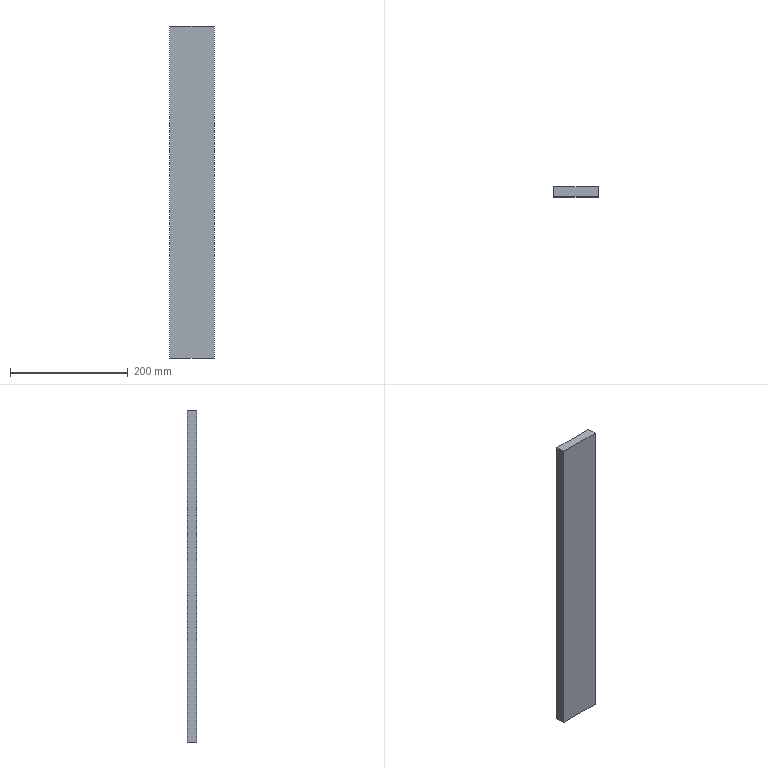Part | SolidWorks | features BaseBody 1 | 1 solid | 6 faces | box 76 x 16 x 563.5 mm | volume 685216 mm3 | plane 6
STEP:
#1=CARTESIAN_POINT('',(53.889,24.883,0.));
#2=VERTEX_POINT('',#1);
#3=CARTESIAN_POINT('',(-22.111,24.883,0.));
#4=VERTEX_POINT('',#3);
#5=CARTESIAN_POINT('',(-22.111,24.883,0.));
#6=DIRECTION('',(-1.,0.,0.));
#7=VECTOR('',#6,1000.);
#8=LINE('',#5,#7);
#9=EDGE_CURVE('',#2,#4,#8,.T.);
#10=ORIENTED_EDGE('',*,*,#9,.T.);
#11=CARTESIAN_POINT('',(-22.111,24.883,563.5));
#12=VERTEX_POINT('',#11);
#13=CARTESIAN_POINT('',(-22.111,24.883,0.));
#14=DIRECTION('',(0.,0.,1.));
#15=VECTOR('',#14,1000.);
#16=LINE('',#13,#15);
#17=EDGE_CURVE('',#4,#12,#16,.T.);
#18=ORIENTED_EDGE('',*,*,#17,.T.);
#19=CARTESIAN_POINT('',(53.889,24.883,563.5));
#20=VERTEX_POINT('',#19);
#21=CARTESIAN_POINT('',(-22.111,24.883,563.5));
#22=DIRECTION('',(1.,0.,0.));
#23=VECTOR('',#22,1000.);
#24=LINE('',#21,#23);
#25=EDGE_CURVE('',#12,#20,#24,.T.);
#26=ORIENTED_EDGE('',*,*,#25,.T.);
#27=CARTESIAN_POINT('',(53.889,24.883,0.));
#28=DIRECTION('',(0.,0.,-1.));
#29=VECTOR('',#28,1000.);
#30=LINE('',#27,#29);
#31=EDGE_CURVE('',#20,#2,#30,.T.);
#32=ORIENTED_EDGE('',*,*,#31,.T.);
#33=EDGE_LOOP('',(#10,#18,#26,#32));
#34=FACE_OUTER_BOUND('',#33,.T.);
#35=CARTESIAN_POINT('',(-22.111,24.883,0.));
#36=DIRECTION('',(0.,1.,0.));
#37=DIRECTION('',(-1.,0.,0.));
#38=AXIS2_PLACEMENT_3D('',#35,#36,#37);
#39=PLANE('',#38);
#40=ADVANCED_FACE('',(#34),#39,.T.);
#41=CARTESIAN_POINT('',(-22.111,8.883,0.));
#42=VERTEX_POINT('',#41);
#43=CARTESIAN_POINT('',(-22.111,8.883,0.));
#44=DIRECTION('',(0.,-1.,0.));
#45=VECTOR('',#44,1000.);
#46=LINE('',#43,#45);
#47=EDGE_CURVE('',#4,#42,#46,.T.);
#48=ORIENTED_EDGE('',*,*,#47,.T.);
#49=CARTESIAN_POINT('',(-22.111,8.883,563.5));
#50=VERTEX_POINT('',#49);
#51=CARTESIAN_POINT('',(-22.111,8.883,0.));
#52=DIRECTION('',(0.,0.,1.));
#53=VECTOR('',#52,1000.);
#54=LINE('',#51,#53);
#55=EDGE_CURVE('',#42,#50,#54,.T.);
#56=ORIENTED_EDGE('',*,*,#55,.T.);
#57=CARTESIAN_POINT('',(-22.111,8.883,563.5));
#58=DIRECTION('',(0.,1.,0.));
#59=VECTOR('',#58,1000.);
#60=LINE('',#57,#59);
#61=EDGE_CURVE('',#50,#12,#60,.T.);
#62=ORIENTED_EDGE('',*,*,#61,.T.);
#63=ORIENTED_EDGE('',*,*,#17,.F.);
#64=EDGE_LOOP('',(#48,#56,#62,#63));
#65=FACE_OUTER_BOUND('',#64,.T.);
#66=CARTESIAN_POINT('',(-22.111,8.883,0.));
#67=DIRECTION('',(-1.,0.,0.));
#68=DIRECTION('',(0.,-1.,0.));
#69=AXIS2_PLACEMENT_3D('',#66,#67,#68);
#70=PLANE('',#69);
#71=ADVANCED_FACE('',(#65),#70,.T.);
#72=CARTESIAN_POINT('',(53.889,8.883,0.));
#73=VERTEX_POINT('',#72);
#74=CARTESIAN_POINT('',(53.889,16.883,0.));
#75=DIRECTION('',(0.,1.,0.));
#76=VECTOR('',#75,1000.);
#77=LINE('',#74,#76);
#78=EDGE_CURVE('',#73,#2,#77,.T.);
#79=ORIENTED_EDGE('',*,*,#78,.F.);
#80=CARTESIAN_POINT('',(15.889,8.883,0.));
#81=DIRECTION('',(1.,0.,0.));
#82=VECTOR('',#81,1000.);
#83=LINE('',#80,#82);
#84=EDGE_CURVE('',#42,#73,#83,.T.);
#85=ORIENTED_EDGE('',*,*,#84,.F.);
#86=ORIENTED_EDGE('',*,*,#47,.F.);
#87=ORIENTED_EDGE('',*,*,#9,.F.);
#88=EDGE_LOOP('',(#79,#85,#86,#87));
#89=FACE_OUTER_BOUND('',#88,.T.);
#90=CARTESIAN_POINT('',(15.889,16.883,0.));
#91=DIRECTION('',(0.,0.,1.));
#92=DIRECTION('',(1.,0.,0.));
#93=AXIS2_PLACEMENT_3D('',#90,#91,#92);
#94=PLANE('',#93);
#95=ADVANCED_FACE('',(#89),#94,.F.);
#96=ORIENTED_EDGE('',*,*,#78,.T.);
#97=ORIENTED_EDGE('',*,*,#31,.F.);
#98=CARTESIAN_POINT('',(53.889,8.883,563.5));
#99=VERTEX_POINT('',#98);
#100=CARTESIAN_POINT('',(53.889,24.883,563.5));
#101=DIRECTION('',(0.,-1.,0.));
#102=VECTOR('',#101,1000.);
#103=LINE('',#100,#102);
#104=EDGE_CURVE('',#20,#99,#103,.T.);
#105=ORIENTED_EDGE('',*,*,#104,.T.);
#106=CARTESIAN_POINT('',(53.889,8.883,0.));
#107=DIRECTION('',(0.,0.,-1.));
#108=VECTOR('',#107,1000.);
#109=LINE('',#106,#108);
#110=EDGE_CURVE('',#99,#73,#109,.T.);
#111=ORIENTED_EDGE('',*,*,#110,.T.);
#112=EDGE_LOOP('',(#96,#97,#105,#111));
#113=FACE_OUTER_BOUND('',#112,.T.);
#114=CARTESIAN_POINT('',(53.889,24.883,0.));
#115=DIRECTION('',(1.,0.,0.));
#116=DIRECTION('',(0.,0.,-1.));
#117=AXIS2_PLACEMENT_3D('',#114,#115,#116);
#118=PLANE('',#117);
#119=ADVANCED_FACE('',(#113),#118,.T.);
#120=ORIENTED_EDGE('',*,*,#61,.F.);
#121=CARTESIAN_POINT('',(15.889,8.883,563.5));
#122=DIRECTION('',(1.,0.,0.));
#123=VECTOR('',#122,1000.);
#124=LINE('',#121,#123);
#125=EDGE_CURVE('',#50,#99,#124,.T.);
#126=ORIENTED_EDGE('',*,*,#125,.T.);
#127=ORIENTED_EDGE('',*,*,#104,.F.);
#128=ORIENTED_EDGE('',*,*,#25,.F.);
#129=EDGE_LOOP('',(#120,#126,#127,#128));
#130=FACE_OUTER_BOUND('',#129,.T.);
#131=CARTESIAN_POINT('',(15.889,16.883,563.5));
#132=DIRECTION('',(0.,0.,1.));
#133=DIRECTION('',(1.,0.,0.));
#134=AXIS2_PLACEMENT_3D('',#131,#132,#133);
#135=PLANE('',#134);
#136=ADVANCED_FACE('',(#130),#135,.T.);
#137=ORIENTED_EDGE('',*,*,#84,.T.);
#138=ORIENTED_EDGE('',*,*,#110,.F.);
#139=ORIENTED_EDGE('',*,*,#125,.F.);
#140=ORIENTED_EDGE('',*,*,#55,.F.);
#141=EDGE_LOOP('',(#137,#138,#139,#140));
#142=FACE_OUTER_BOUND('',#141,.T.);
#143=CARTESIAN_POINT('',(53.889,8.883,0.));
#144=DIRECTION('',(0.,-1.,0.));
#145=DIRECTION('',(1.,0.,0.));
#146=AXIS2_PLACEMENT_3D('',#143,#144,#145);
#147=PLANE('',#146);
#148=ADVANCED_FACE('',(#142),#147,.T.);
#149=CLOSED_SHELL('',(#40,#71,#95,#119,#136,#148));
#150=MANIFOLD_SOLID_BREP('',#149);
#151=CARTESIAN_POINT('',(0.,0.,0.));
#152=DIRECTION('',(0.,0.,1.));
#153=DIRECTION('',(1.,0.,0.));
#154=AXIS2_PLACEMENT_3D('',#151,#152,#153);
#155=(LENGTH_UNIT()NAMED_UNIT(*)SI_UNIT(.MILLI.,.METRE.));
#156=UNCERTAINTY_MEASURE_WITH_UNIT(LENGTH_MEASURE(0.00001),#155,'','');
#157=(NAMED_UNIT(*)PLANE_ANGLE_UNIT()SI_UNIT($,.RADIAN.));
#158=(NAMED_UNIT(*)SI_UNIT($,.STERADIAN.)SOLID_ANGLE_UNIT());
#159=(GEOMETRIC_REPRESENTATION_CONTEXT(3)GLOBAL_UNCERTAINTY_ASSIGNED_CONTEXT((#156))GLOBAL_UNIT_ASSIGNED_CONTEXT((#155,#157,#158))REPRESENTATION_CONTEXT('',''));
#160=ADVANCED_BREP_SHAPE_REPRESENTATION('',(#150,#154),#159);